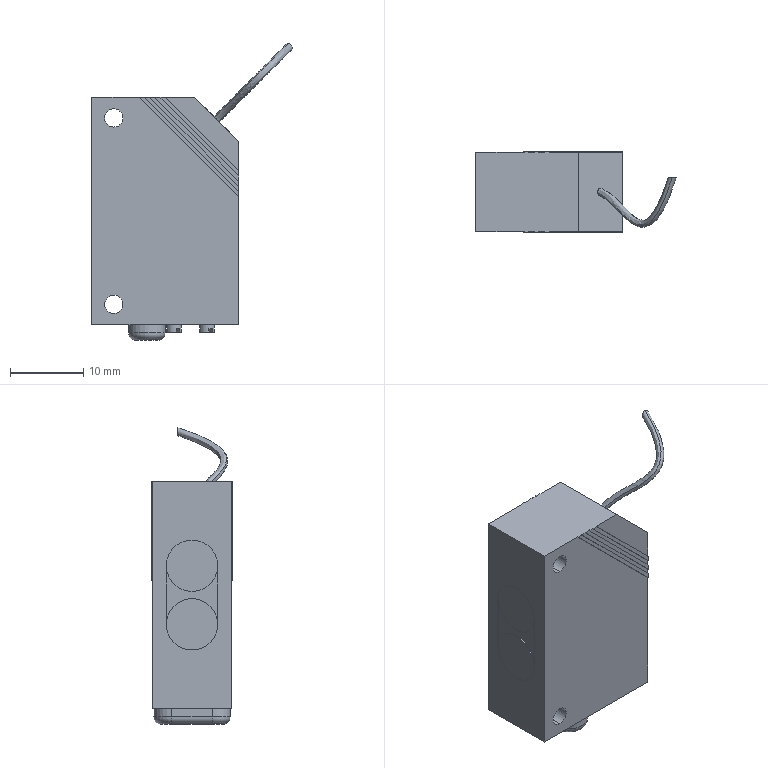Part | SolidWorks | features ICE 6, 3DProfileFeature 2, Chamfer 1, Extrusion 1, Fillet 1, HoleWzd 1, MirrorPattern 1, Sweep 1 | 1 solid | 72 faces | box 27.316 x 11 x 40.416 mm | volume 6512 mm3 | plane 50 | cylinder 18 | spline 2 | torus 2 | commonest cylinder face diameters 2 x6 7 x6 2.5 x4 5 x2